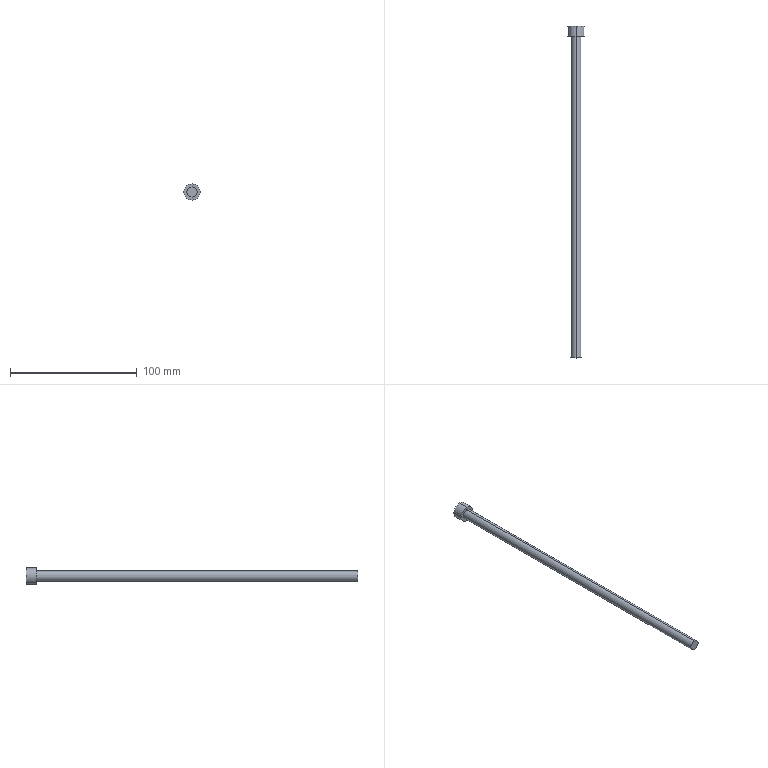Part | STEP file | 1 solid | 7 faces | box 13 x 262.36 x 13 mm | volume 13847 mm3 | cylinder 4 | plane 3 | commonest cylinder face diameters 8 x2 13 x2
STEP:
#1=CARTESIAN_POINT('',(0.,0.,0.));
#2=DIRECTION('',(0.,0.,1.));
#3=DIRECTION('',(1.,0.,0.));
#4=AXIS2_PLACEMENT_3D('',#1,#2,#3);
#5=CARTESIAN_POINT('',(-115.86,290.5,187.029));
#6=VERTEX_POINT('',#5);
#7=CARTESIAN_POINT('',(-115.86,290.5,200.029));
#8=VERTEX_POINT('',#7);
#9=CARTESIAN_POINT('',(-115.86,290.5,193.529));
#10=DIRECTION('',(0.,-1.,0.));
#11=DIRECTION('',(0.,0.,-1.));
#12=AXIS2_PLACEMENT_3D('',#9,#10,#11);
#13=CIRCLE('',#12,6.5);
#14=CARTESIAN_POINT('',(-115.86,290.5,193.529));
#15=DIRECTION('',(0.,-1.,0.));
#16=DIRECTION('',(0.,0.,-1.));
#17=AXIS2_PLACEMENT_3D('',#14,#15,#16);
#18=CYLINDRICAL_SURFACE('',#17,6.5);
#19=CARTESIAN_POINT('',(0.,0.));
#20=DIRECTION('',(1.,0.));
#21=VECTOR('',#20,1.);
#22=LINE('',#19,#21);
#23=(GEOMETRIC_REPRESENTATION_CONTEXT(2)PARAMETRIC_REPRESENTATION_CONTEXT()REPRESENTATION_CONTEXT('',''));
#24=DEFINITIONAL_REPRESENTATION('',(#22),#23);
#25=PCURVE('',#18,#24);
#26=CARTESIAN_POINT('',(-72.862,290.5,110.196));
#27=DIRECTION('',(0.,-1.,0.));
#28=DIRECTION('',(0.,0.,-1.));
#29=AXIS2_PLACEMENT_3D('',#26,#27,#28);
#30=PLANE('',#29);
#31=CARTESIAN_POINT('',(-83.333,-42.997));
#32=DIRECTION('',(1.,0.));
#33=AXIS2_PLACEMENT_2D('',#31,#32);
#34=CIRCLE('',#33,6.5);
#35=(GEOMETRIC_REPRESENTATION_CONTEXT(2)PARAMETRIC_REPRESENTATION_CONTEXT()REPRESENTATION_CONTEXT('',''));
#36=DEFINITIONAL_REPRESENTATION('',(#34),#35);
#37=PCURVE('',#30,#36);
#38=SURFACE_CURVE('',#13,(#25,#37),.PCURVE_S1.);
#39=EDGE_CURVE('',#6,#8,#38,.T.);
#40=ORIENTED_EDGE('',*,*,#39,.T.);
#41=CARTESIAN_POINT('',(-115.86,282.5,200.029));
#42=VERTEX_POINT('',#41);
#43=CARTESIAN_POINT('',(-115.86,290.5,200.029));
#44=DIRECTION('',(0.,-1.,0.));
#45=VECTOR('',#44,1.);
#46=LINE('',#43,#45);
#47=CARTESIAN_POINT('',(3.142,0.));
#48=DIRECTION('',(0.,1.));
#49=VECTOR('',#48,1.);
#50=LINE('',#47,#49);
#51=(GEOMETRIC_REPRESENTATION_CONTEXT(2)PARAMETRIC_REPRESENTATION_CONTEXT()REPRESENTATION_CONTEXT('',''));
#52=DEFINITIONAL_REPRESENTATION('',(#50),#51);
#53=PCURVE('',#18,#52);
#54=CARTESIAN_POINT('',(-115.86,290.5,193.529));
#55=DIRECTION('',(0.,-1.,0.));
#56=DIRECTION('',(0.,0.,-1.));
#57=AXIS2_PLACEMENT_3D('',#54,#55,#56);
#58=CYLINDRICAL_SURFACE('',#57,6.5);
#59=CARTESIAN_POINT('',(3.142,0.));
#60=DIRECTION('',(0.,1.));
#61=VECTOR('',#60,1.);
#62=LINE('',#59,#61);
#63=(GEOMETRIC_REPRESENTATION_CONTEXT(2)PARAMETRIC_REPRESENTATION_CONTEXT()REPRESENTATION_CONTEXT('',''));
#64=DEFINITIONAL_REPRESENTATION('',(#62),#63);
#65=PCURVE('',#58,#64);
#66=SURFACE_CURVE('',#46,(#53,#65),.PCURVE_S1.);
#67=EDGE_CURVE('',#8,#42,#66,.T.);
#68=ORIENTED_EDGE('',*,*,#67,.T.);
#69=CARTESIAN_POINT('',(-115.86,282.5,187.029));
#70=VERTEX_POINT('',#69);
#71=CARTESIAN_POINT('',(-115.86,282.5,193.529));
#72=DIRECTION('',(0.,1.,0.));
#73=DIRECTION('',(0.,0.,1.));
#74=AXIS2_PLACEMENT_3D('',#71,#72,#73);
#75=CIRCLE('',#74,6.5);
#76=CARTESIAN_POINT('',(3.142,8.));
#77=DIRECTION('',(-1.,0.));
#78=VECTOR('',#77,1.);
#79=LINE('',#76,#78);
#80=(GEOMETRIC_REPRESENTATION_CONTEXT(2)PARAMETRIC_REPRESENTATION_CONTEXT()REPRESENTATION_CONTEXT('',''));
#81=DEFINITIONAL_REPRESENTATION('',(#79),#80);
#82=PCURVE('',#18,#81);
#83=CARTESIAN_POINT('',(-115.86,282.5,193.529));
#84=DIRECTION('',(0.,-1.,0.));
#85=DIRECTION('',(0.,0.,-1.));
#86=AXIS2_PLACEMENT_3D('',#83,#84,#85);
#87=PLANE('',#86);
#88=CARTESIAN_POINT('',(-6.5,0.));
#89=CARTESIAN_POINT('',(-6.5,11.258));
#90=CARTESIAN_POINT('',(3.25,5.629));
#91=CARTESIAN_POINT('',(13.,0.));
#92=CARTESIAN_POINT('',(3.25,-5.629));
#93=CARTESIAN_POINT('',(-6.5,-11.258));
#94=CARTESIAN_POINT('',(-6.5,0.));
#95=(BOUNDED_CURVE()B_SPLINE_CURVE(2,(#88,#89,#90,#91,#92,#93,#94),.UNSPECIFIED.,.T.,.F.)B_SPLINE_CURVE_WITH_KNOTS((1,2,2,2,2,1),(-2.094,0.,2.094,4.189,6.283,8.378),.UNSPECIFIED.)CURVE()GEOMETRIC_REPRESENTATION_ITEM()RATIONAL_B_SPLINE_CURVE((1.,0.5,1.,0.5,1.,0.5,1.))REPRESENTATION_ITEM(''));
#96=(GEOMETRIC_REPRESENTATION_CONTEXT(2)PARAMETRIC_REPRESENTATION_CONTEXT()REPRESENTATION_CONTEXT('',''));
#97=DEFINITIONAL_REPRESENTATION('',(#95),#96);
#98=PCURVE('',#87,#97);
#99=SURFACE_CURVE('',#75,(#82,#98),.PCURVE_S1.);
#100=EDGE_CURVE('',#42,#70,#99,.T.);
#101=ORIENTED_EDGE('',*,*,#100,.T.);
#102=CARTESIAN_POINT('',(-115.86,290.5,187.029));
#103=DIRECTION('',(0.,-1.,0.));
#104=VECTOR('',#103,1.);
#105=LINE('',#102,#104);
#106=CARTESIAN_POINT('',(0.,0.));
#107=DIRECTION('',(0.,1.));
#108=VECTOR('',#107,1.);
#109=LINE('',#106,#108);
#110=(GEOMETRIC_REPRESENTATION_CONTEXT(2)PARAMETRIC_REPRESENTATION_CONTEXT()REPRESENTATION_CONTEXT('',''));
#111=DEFINITIONAL_REPRESENTATION('',(#109),#110);
#112=PCURVE('',#18,#111);
#113=CARTESIAN_POINT('',(6.283,0.));
#114=DIRECTION('',(0.,1.));
#115=VECTOR('',#114,1.);
#116=LINE('',#113,#115);
#117=(GEOMETRIC_REPRESENTATION_CONTEXT(2)PARAMETRIC_REPRESENTATION_CONTEXT()REPRESENTATION_CONTEXT('',''));
#118=DEFINITIONAL_REPRESENTATION('',(#116),#117);
#119=PCURVE('',#58,#118);
#120=SURFACE_CURVE('',#105,(#112,#119),.PCURVE_S1.);
#121=EDGE_CURVE('',#6,#70,#120,.T.);
#122=ORIENTED_EDGE('',*,*,#121,.F.);
#123=EDGE_LOOP('',(#40,#68,#101,#122));
#124=FACE_BOUND('',#123,.T.);
#125=ADVANCED_FACE('',(#124),#18,.T.);
#126=CARTESIAN_POINT('',(-115.86,282.5,197.529));
#127=VERTEX_POINT('',#126);
#128=CARTESIAN_POINT('',(-115.86,282.5,189.529));
#129=VERTEX_POINT('',#128);
#130=CARTESIAN_POINT('',(-115.86,282.5,193.529));
#131=DIRECTION('',(0.,1.,0.));
#132=DIRECTION('',(0.,0.,-1.));
#133=AXIS2_PLACEMENT_3D('',#130,#131,#132);
#134=CIRCLE('',#133,4.);
#135=CARTESIAN_POINT('',(-115.86,220.5,193.529));
#136=DIRECTION('',(0.,-1.,0.));
#137=DIRECTION('',(0.,0.,-1.));
#138=AXIS2_PLACEMENT_3D('',#135,#136,#137);
#139=CYLINDRICAL_SURFACE('',#138,4.);
#140=CARTESIAN_POINT('',(6.283,-62.));
#141=DIRECTION('',(-1.,0.));
#142=VECTOR('',#141,1.);
#143=LINE('',#140,#142);
#144=(GEOMETRIC_REPRESENTATION_CONTEXT(2)PARAMETRIC_REPRESENTATION_CONTEXT()REPRESENTATION_CONTEXT('',''));
#145=DEFINITIONAL_REPRESENTATION('',(#143),#144);
#146=PCURVE('',#139,#145);
#147=CARTESIAN_POINT('',(4.,0.));
#148=CARTESIAN_POINT('',(4.,-6.928));
#149=CARTESIAN_POINT('',(-2.,-3.464));
#150=CARTESIAN_POINT('',(-8.,0.));
#151=CARTESIAN_POINT('',(-2.,3.464));
#152=CARTESIAN_POINT('',(4.,6.928));
#153=CARTESIAN_POINT('',(4.,0.));
#154=(BOUNDED_CURVE()B_SPLINE_CURVE(2,(#147,#148,#149,#150,#151,#152,#153),.UNSPECIFIED.,.T.,.F.)B_SPLINE_CURVE_WITH_KNOTS((1,2,2,2,2,1),(-2.094,0.,2.094,4.189,6.283,8.378),.UNSPECIFIED.)CURVE()GEOMETRIC_REPRESENTATION_ITEM()RATIONAL_B_SPLINE_CURVE((1.,0.5,1.,0.5,1.,0.5,1.))REPRESENTATION_ITEM(''));
#155=(GEOMETRIC_REPRESENTATION_CONTEXT(2)PARAMETRIC_REPRESENTATION_CONTEXT()REPRESENTATION_CONTEXT('',''));
#156=DEFINITIONAL_REPRESENTATION('',(#154),#155);
#157=PCURVE('',#87,#156);
#158=SURFACE_CURVE('',#134,(#146,#157),.PCURVE_S1.);
#159=EDGE_CURVE('',#127,#129,#158,.T.);
#160=ORIENTED_EDGE('',*,*,#159,.F.);
#161=CARTESIAN_POINT('',(-115.86,28.14,197.529));
#162=VERTEX_POINT('',#161);
#163=CARTESIAN_POINT('',(-115.86,220.5,197.529));
#164=DIRECTION('',(0.,-1.,0.));
#165=VECTOR('',#164,1.);
#166=LINE('',#163,#165);
#167=CARTESIAN_POINT('',(3.142,0.));
#168=DIRECTION('',(0.,1.));
#169=VECTOR('',#168,1.);
#170=LINE('',#167,#169);
#171=(GEOMETRIC_REPRESENTATION_CONTEXT(2)PARAMETRIC_REPRESENTATION_CONTEXT()REPRESENTATION_CONTEXT('',''));
#172=DEFINITIONAL_REPRESENTATION('',(#170),#171);
#173=PCURVE('',#139,#172);
#174=CARTESIAN_POINT('',(-115.86,220.5,193.529));
#175=DIRECTION('',(0.,-1.,0.));
#176=DIRECTION('',(0.,0.,-1.));
#177=AXIS2_PLACEMENT_3D('',#174,#175,#176);
#178=CYLINDRICAL_SURFACE('',#177,4.);
#179=CARTESIAN_POINT('',(3.142,0.));
#180=DIRECTION('',(0.,1.));
#181=VECTOR('',#180,1.);
#182=LINE('',#179,#181);
#183=(GEOMETRIC_REPRESENTATION_CONTEXT(2)PARAMETRIC_REPRESENTATION_CONTEXT()REPRESENTATION_CONTEXT('',''));
#184=DEFINITIONAL_REPRESENTATION('',(#182),#183);
#185=PCURVE('',#178,#184);
#186=SURFACE_CURVE('',#166,(#173,#185),.PCURVE_S1.);
#187=EDGE_CURVE('',#127,#162,#186,.T.);
#188=ORIENTED_EDGE('',*,*,#187,.T.);
#189=CARTESIAN_POINT('',(-115.86,28.14,189.529));
#190=VERTEX_POINT('',#189);
#191=CARTESIAN_POINT('',(-115.86,28.14,193.529));
#192=DIRECTION('',(0.,1.,0.));
#193=DIRECTION('',(0.,0.,-1.));
#194=AXIS2_PLACEMENT_3D('',#191,#192,#193);
#195=CIRCLE('',#194,4.);
#196=CARTESIAN_POINT('',(6.283,192.36));
#197=DIRECTION('',(-1.,0.));
#198=VECTOR('',#197,1.);
#199=LINE('',#196,#198);
#200=(GEOMETRIC_REPRESENTATION_CONTEXT(2)PARAMETRIC_REPRESENTATION_CONTEXT()REPRESENTATION_CONTEXT('',''));
#201=DEFINITIONAL_REPRESENTATION('',(#199),#200);
#202=PCURVE('',#139,#201);
#203=CARTESIAN_POINT('',(-72.862,28.14,-91.563));
#204=DIRECTION('',(0.,-1.,0.));
#205=DIRECTION('',(0.,0.,-1.));
#206=AXIS2_PLACEMENT_3D('',#203,#204,#205);
#207=PLANE('',#206);
#208=CARTESIAN_POINT('',(-281.093,-42.997));
#209=CARTESIAN_POINT('',(-281.093,-49.926));
#210=CARTESIAN_POINT('',(-287.093,-46.461));
#211=CARTESIAN_POINT('',(-293.093,-42.997));
#212=CARTESIAN_POINT('',(-287.093,-39.533));
#213=CARTESIAN_POINT('',(-281.093,-36.069));
#214=CARTESIAN_POINT('',(-281.093,-42.997));
#215=(BOUNDED_CURVE()B_SPLINE_CURVE(2,(#208,#209,#210,#211,#212,#213,#214),.UNSPECIFIED.,.T.,.F.)B_SPLINE_CURVE_WITH_KNOTS((1,2,2,2,2,1),(-2.094,0.,2.094,4.189,6.283,8.378),.UNSPECIFIED.)CURVE()GEOMETRIC_REPRESENTATION_ITEM()RATIONAL_B_SPLINE_CURVE((1.,0.5,1.,0.5,1.,0.5,1.))REPRESENTATION_ITEM(''));
#216=(GEOMETRIC_REPRESENTATION_CONTEXT(2)PARAMETRIC_REPRESENTATION_CONTEXT()REPRESENTATION_CONTEXT('',''));
#217=DEFINITIONAL_REPRESENTATION('',(#215),#216);
#218=PCURVE('',#207,#217);
#219=SURFACE_CURVE('',#195,(#202,#218),.PCURVE_S1.);
#220=EDGE_CURVE('',#162,#190,#219,.T.);
#221=ORIENTED_EDGE('',*,*,#220,.T.);
#222=CARTESIAN_POINT('',(-115.86,220.5,189.529));
#223=DIRECTION('',(0.,-1.,0.));
#224=VECTOR('',#223,1.);
#225=LINE('',#222,#224);
#226=CARTESIAN_POINT('',(0.,0.));
#227=DIRECTION('',(0.,1.));
#228=VECTOR('',#227,1.);
#229=LINE('',#226,#228);
#230=(GEOMETRIC_REPRESENTATION_CONTEXT(2)PARAMETRIC_REPRESENTATION_CONTEXT()REPRESENTATION_CONTEXT('',''));
#231=DEFINITIONAL_REPRESENTATION('',(#229),#230);
#232=PCURVE('',#139,#231);
#233=CARTESIAN_POINT('',(6.283,0.));
#234=DIRECTION('',(0.,1.));
#235=VECTOR('',#234,1.);
#236=LINE('',#233,#235);
#237=(GEOMETRIC_REPRESENTATION_CONTEXT(2)PARAMETRIC_REPRESENTATION_CONTEXT()REPRESENTATION_CONTEXT('',''));
#238=DEFINITIONAL_REPRESENTATION('',(#236),#237);
#239=PCURVE('',#178,#238);
#240=SURFACE_CURVE('',#225,(#232,#239),.PCURVE_S1.);
#241=EDGE_CURVE('',#129,#190,#240,.T.);
#242=ORIENTED_EDGE('',*,*,#241,.F.);
#243=EDGE_LOOP('',(#160,#188,#221,#242));
#244=FACE_BOUND('',#243,.T.);
#245=ADVANCED_FACE('',(#244),#139,.T.);
#246=ORIENTED_EDGE('',*,*,#187,.F.);
#247=CARTESIAN_POINT('',(-115.86,282.5,193.529));
#248=DIRECTION('',(0.,1.,0.));
#249=DIRECTION('',(0.,0.,-1.));
#250=AXIS2_PLACEMENT_3D('',#247,#248,#249);
#251=CIRCLE('',#250,4.);
#252=CARTESIAN_POINT('',(6.283,-62.));
#253=DIRECTION('',(-1.,0.));
#254=VECTOR('',#253,1.);
#255=LINE('',#252,#254);
#256=(GEOMETRIC_REPRESENTATION_CONTEXT(2)PARAMETRIC_REPRESENTATION_CONTEXT()REPRESENTATION_CONTEXT('',''));
#257=DEFINITIONAL_REPRESENTATION('',(#255),#256);
#258=PCURVE('',#178,#257);
#259=CARTESIAN_POINT('',(4.,0.));
#260=CARTESIAN_POINT('',(4.,-6.928));
#261=CARTESIAN_POINT('',(-2.,-3.464));
#262=CARTESIAN_POINT('',(-8.,0.));
#263=CARTESIAN_POINT('',(-2.,3.464));
#264=CARTESIAN_POINT('',(4.,6.928));
#265=CARTESIAN_POINT('',(4.,0.));
#266=(BOUNDED_CURVE()B_SPLINE_CURVE(2,(#259,#260,#261,#262,#263,#264,#265),.UNSPECIFIED.,.T.,.F.)B_SPLINE_CURVE_WITH_KNOTS((1,2,2,2,2,1),(-2.094,0.,2.094,4.189,6.283,8.378),.UNSPECIFIED.)CURVE()GEOMETRIC_REPRESENTATION_ITEM()RATIONAL_B_SPLINE_CURVE((1.,0.5,1.,0.5,1.,0.5,1.))REPRESENTATION_ITEM(''));
#267=(GEOMETRIC_REPRESENTATION_CONTEXT(2)PARAMETRIC_REPRESENTATION_CONTEXT()REPRESENTATION_CONTEXT('',''));
#268=DEFINITIONAL_REPRESENTATION('',(#266),#267);
#269=PCURVE('',#87,#268);
#270=SURFACE_CURVE('',#251,(#258,#269),.PCURVE_S1.);
#271=EDGE_CURVE('',#129,#127,#270,.T.);
#272=ORIENTED_EDGE('',*,*,#271,.F.);
#273=ORIENTED_EDGE('',*,*,#241,.T.);
#274=CARTESIAN_POINT('',(-115.86,28.14,193.529));
#275=DIRECTION('',(0.,1.,0.));
#276=DIRECTION('',(0.,0.,-1.));
#277=AXIS2_PLACEMENT_3D('',#274,#275,#276);
#278=CIRCLE('',#277,4.);
#279=CARTESIAN_POINT('',(6.283,192.36));
#280=DIRECTION('',(-1.,0.));
#281=VECTOR('',#280,1.);
#282=LINE('',#279,#281);
#283=(GEOMETRIC_REPRESENTATION_CONTEXT(2)PARAMETRIC_REPRESENTATION_CONTEXT()REPRESENTATION_CONTEXT('',''));
#284=DEFINITIONAL_REPRESENTATION('',(#282),#283);
#285=PCURVE('',#178,#284);
#286=CARTESIAN_POINT('',(-281.093,-42.997));
#287=CARTESIAN_POINT('',(-281.093,-49.926));
#288=CARTESIAN_POINT('',(-287.093,-46.461));
#289=CARTESIAN_POINT('',(-293.093,-42.997));
#290=CARTESIAN_POINT('',(-287.093,-39.533));
#291=CARTESIAN_POINT('',(-281.093,-36.069));
#292=CARTESIAN_POINT('',(-281.093,-42.997));
#293=(BOUNDED_CURVE()B_SPLINE_CURVE(2,(#286,#287,#288,#289,#290,#291,#292),.UNSPECIFIED.,.T.,.F.)B_SPLINE_CURVE_WITH_KNOTS((1,2,2,2,2,1),(-2.094,0.,2.094,4.189,6.283,8.378),.UNSPECIFIED.)CURVE()GEOMETRIC_REPRESENTATION_ITEM()RATIONAL_B_SPLINE_CURVE((1.,0.5,1.,0.5,1.,0.5,1.))REPRESENTATION_ITEM(''));
#294=(GEOMETRIC_REPRESENTATION_CONTEXT(2)PARAMETRIC_REPRESENTATION_CONTEXT()REPRESENTATION_CONTEXT('',''));
#295=DEFINITIONAL_REPRESENTATION('',(#293),#294);
#296=PCURVE('',#207,#295);
#297=SURFACE_CURVE('',#278,(#285,#296),.PCURVE_S1.);
#298=EDGE_CURVE('',#190,#162,#297,.T.);
#299=ORIENTED_EDGE('',*,*,#298,.T.);
#300=EDGE_LOOP('',(#246,#272,#273,#299));
#301=FACE_BOUND('',#300,.T.);
#302=ADVANCED_FACE('',(#301),#178,.T.);
#303=ORIENTED_EDGE('',*,*,#298,.F.);
#304=ORIENTED_EDGE('',*,*,#220,.F.);
#305=EDGE_LOOP('',(#303,#304));
#306=FACE_BOUND('',#305,.T.);
#307=ADVANCED_FACE('',(#306),#207,.T.);
#308=ORIENTED_EDGE('',*,*,#271,.T.);
#309=ORIENTED_EDGE('',*,*,#159,.T.);
#310=EDGE_LOOP('',(#308,#309));
#311=FACE_BOUND('',#310,.T.);
#312=CARTESIAN_POINT('',(-115.86,282.5,193.529));
#313=DIRECTION('',(0.,1.,0.));
#314=DIRECTION('',(0.,0.,1.));
#315=AXIS2_PLACEMENT_3D('',#312,#313,#314);
#316=CIRCLE('',#315,6.5);
#317=CARTESIAN_POINT('',(-6.5,0.));
#318=CARTESIAN_POINT('',(-6.5,11.258));
#319=CARTESIAN_POINT('',(3.25,5.629));
#320=CARTESIAN_POINT('',(13.,0.));
#321=CARTESIAN_POINT('',(3.25,-5.629));
#322=CARTESIAN_POINT('',(-6.5,-11.258));
#323=CARTESIAN_POINT('',(-6.5,0.));
#324=(BOUNDED_CURVE()B_SPLINE_CURVE(2,(#317,#318,#319,#320,#321,#322,#323),.UNSPECIFIED.,.T.,.F.)B_SPLINE_CURVE_WITH_KNOTS((1,2,2,2,2,1),(-2.094,0.,2.094,4.189,6.283,8.378),.UNSPECIFIED.)CURVE()GEOMETRIC_REPRESENTATION_ITEM()RATIONAL_B_SPLINE_CURVE((1.,0.5,1.,0.5,1.,0.5,1.))REPRESENTATION_ITEM(''));
#325=(GEOMETRIC_REPRESENTATION_CONTEXT(2)PARAMETRIC_REPRESENTATION_CONTEXT()REPRESENTATION_CONTEXT('',''));
#326=DEFINITIONAL_REPRESENTATION('',(#324),#325);
#327=PCURVE('',#87,#326);
#328=CARTESIAN_POINT('',(9.425,8.));
#329=DIRECTION('',(-1.,0.));
#330=VECTOR('',#329,1.);
#331=LINE('',#328,#330);
#332=(GEOMETRIC_REPRESENTATION_CONTEXT(2)PARAMETRIC_REPRESENTATION_CONTEXT()REPRESENTATION_CONTEXT('',''));
#333=DEFINITIONAL_REPRESENTATION('',(#331),#332);
#334=PCURVE('',#58,#333);
#335=SURFACE_CURVE('',#316,(#327,#334),.PCURVE_S1.);
#336=EDGE_CURVE('',#70,#42,#335,.T.);
#337=ORIENTED_EDGE('',*,*,#336,.F.);
#338=ORIENTED_EDGE('',*,*,#100,.F.);
#339=EDGE_LOOP('',(#337,#338));
#340=FACE_BOUND('',#339,.T.);
#341=ADVANCED_FACE('',(#311,#340),#87,.T.);
#342=ORIENTED_EDGE('',*,*,#67,.F.);
#343=CARTESIAN_POINT('',(-115.86,290.5,193.529));
#344=DIRECTION('',(0.,-1.,0.));
#345=DIRECTION('',(0.,0.,-1.));
#346=AXIS2_PLACEMENT_3D('',#343,#344,#345);
#347=CIRCLE('',#346,6.5);
#348=CARTESIAN_POINT('',(0.,0.));
#349=DIRECTION('',(1.,0.));
#350=VECTOR('',#349,1.);
#351=LINE('',#348,#350);
#352=(GEOMETRIC_REPRESENTATION_CONTEXT(2)PARAMETRIC_REPRESENTATION_CONTEXT()REPRESENTATION_CONTEXT('',''));
#353=DEFINITIONAL_REPRESENTATION('',(#351),#352);
#354=PCURVE('',#58,#353);
#355=CARTESIAN_POINT('',(-83.333,-42.997));
#356=DIRECTION('',(1.,0.));
#357=AXIS2_PLACEMENT_2D('',#355,#356);
#358=CIRCLE('',#357,6.5);
#359=(GEOMETRIC_REPRESENTATION_CONTEXT(2)PARAMETRIC_REPRESENTATION_CONTEXT()REPRESENTATION_CONTEXT('',''));
#360=DEFINITIONAL_REPRESENTATION('',(#358),#359);
#361=PCURVE('',#30,#360);
#362=SURFACE_CURVE('',#347,(#354,#361),.PCURVE_S1.);
#363=EDGE_CURVE('',#8,#6,#362,.T.);
#364=ORIENTED_EDGE('',*,*,#363,.T.);
#365=ORIENTED_EDGE('',*,*,#121,.T.);
#366=ORIENTED_EDGE('',*,*,#336,.T.);
#367=EDGE_LOOP('',(#342,#364,#365,#366));
#368=FACE_BOUND('',#367,.T.);
#369=ADVANCED_FACE('',(#368),#58,.T.);
#370=ORIENTED_EDGE('',*,*,#39,.F.);
#371=ORIENTED_EDGE('',*,*,#363,.F.);
#372=EDGE_LOOP('',(#370,#371));
#373=FACE_BOUND('',#372,.T.);
#374=ADVANCED_FACE('',(#373),#30,.F.);
#375=CLOSED_SHELL('',(#125,#245,#302,#307,#341,#369,#374));
#376=MANIFOLD_SOLID_BREP('',#375);
#377=(LENGTH_UNIT()NAMED_UNIT(*)SI_UNIT(.MILLI.,.METRE.));
#378=UNCERTAINTY_MEASURE_WITH_UNIT(LENGTH_MEASURE(0.0000001),#377,'','');
#379=(NAMED_UNIT(*)PLANE_ANGLE_UNIT()SI_UNIT($,.RADIAN.));
#380=(NAMED_UNIT(*)SI_UNIT($,.STERADIAN.)SOLID_ANGLE_UNIT());
#381=(GEOMETRIC_REPRESENTATION_CONTEXT(3)GLOBAL_UNCERTAINTY_ASSIGNED_CONTEXT((#378))GLOBAL_UNIT_ASSIGNED_CONTEXT((#377,#379,#380))REPRESENTATION_CONTEXT('',''));
#382=ADVANCED_BREP_SHAPE_REPRESENTATION('',(#4,#376),#381);